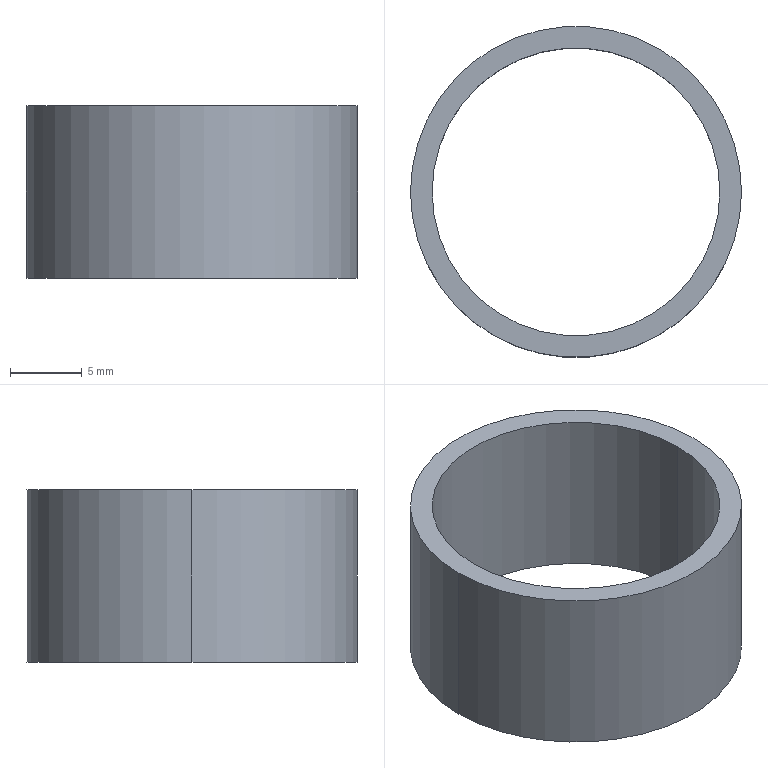Part | SolidWorks | features Extrusion 1 | 1 solid | 6 faces | box 23 x 23 x 12 mm | volume 1216 mm3 | cylinder 4 | plane 2 | commonest cylinder face diameters 20 x2 23 x2
STEP:
#1=CARTESIAN_POINT('',(-10.,0.,12.));
#2=VERTEX_POINT('',#1);
#3=CARTESIAN_POINT('',(10.,0.,12.));
#4=VERTEX_POINT('',#3);
#5=CARTESIAN_POINT('',(0.,0.,12.));
#6=DIRECTION('',(0.,0.,1.));
#7=DIRECTION('',(1.,0.,0.));
#8=AXIS2_PLACEMENT_3D('',#5,#6,#7);
#9=CIRCLE('',#8,10.);
#10=EDGE_CURVE('',#2,#4,#9,.T.);
#11=ORIENTED_EDGE('',*,*,#10,.T.);
#12=CARTESIAN_POINT('',(10.,0.,0.));
#13=VERTEX_POINT('',#12);
#14=CARTESIAN_POINT('',(10.,0.,12.));
#15=DIRECTION('',(0.,0.,-1.));
#16=VECTOR('',#15,1000.);
#17=LINE('',#14,#16);
#18=EDGE_CURVE('',#4,#13,#17,.T.);
#19=ORIENTED_EDGE('',*,*,#18,.T.);
#20=CARTESIAN_POINT('',(-10.,0.,0.));
#21=VERTEX_POINT('',#20);
#22=CARTESIAN_POINT('',(0.,0.,0.));
#23=DIRECTION('',(0.,0.,1.));
#24=DIRECTION('',(1.,0.,0.));
#25=AXIS2_PLACEMENT_3D('',#22,#23,#24);
#26=CIRCLE('',#25,10.);
#27=EDGE_CURVE('',#21,#13,#26,.T.);
#28=ORIENTED_EDGE('',*,*,#27,.F.);
#29=CARTESIAN_POINT('',(-10.,0.,12.));
#30=DIRECTION('',(0.,0.,-1.));
#31=VECTOR('',#30,1000.);
#32=LINE('',#29,#31);
#33=EDGE_CURVE('',#2,#21,#32,.T.);
#34=ORIENTED_EDGE('',*,*,#33,.F.);
#35=EDGE_LOOP('',(#11,#19,#28,#34));
#36=FACE_OUTER_BOUND('',#35,.T.);
#37=CARTESIAN_POINT('',(0.,0.,12.));
#38=DIRECTION('',(0.,0.,-1.));
#39=DIRECTION('',(-1.,0.,0.));
#40=AXIS2_PLACEMENT_3D('',#37,#38,#39);
#41=CYLINDRICAL_SURFACE('',#40,10.);
#42=ADVANCED_FACE('',(#36),#41,.F.);
#43=CARTESIAN_POINT('',(11.5,0.,12.));
#44=VERTEX_POINT('',#43);
#45=CARTESIAN_POINT('',(-11.5,0.,12.));
#46=VERTEX_POINT('',#45);
#47=CARTESIAN_POINT('',(0.,0.,12.));
#48=DIRECTION('',(0.,0.,1.));
#49=DIRECTION('',(1.,0.,0.));
#50=AXIS2_PLACEMENT_3D('',#47,#48,#49);
#51=CIRCLE('',#50,11.5);
#52=EDGE_CURVE('',#44,#46,#51,.T.);
#53=ORIENTED_EDGE('',*,*,#52,.F.);
#54=CARTESIAN_POINT('',(11.5,0.,0.));
#55=VERTEX_POINT('',#54);
#56=CARTESIAN_POINT('',(11.5,0.,12.));
#57=DIRECTION('',(0.,0.,-1.));
#58=VECTOR('',#57,1000.);
#59=LINE('',#56,#58);
#60=EDGE_CURVE('',#44,#55,#59,.T.);
#61=ORIENTED_EDGE('',*,*,#60,.T.);
#62=CARTESIAN_POINT('',(-11.5,0.,0.));
#63=VERTEX_POINT('',#62);
#64=CARTESIAN_POINT('',(0.,0.,0.));
#65=DIRECTION('',(0.,0.,1.));
#66=DIRECTION('',(1.,0.,0.));
#67=AXIS2_PLACEMENT_3D('',#64,#65,#66);
#68=CIRCLE('',#67,11.5);
#69=EDGE_CURVE('',#55,#63,#68,.T.);
#70=ORIENTED_EDGE('',*,*,#69,.T.);
#71=CARTESIAN_POINT('',(-11.5,0.,12.));
#72=DIRECTION('',(0.,0.,-1.));
#73=VECTOR('',#72,1000.);
#74=LINE('',#71,#73);
#75=EDGE_CURVE('',#46,#63,#74,.T.);
#76=ORIENTED_EDGE('',*,*,#75,.F.);
#77=EDGE_LOOP('',(#53,#61,#70,#76));
#78=FACE_OUTER_BOUND('',#77,.T.);
#79=CARTESIAN_POINT('',(0.,0.,12.));
#80=DIRECTION('',(0.,0.,-1.));
#81=DIRECTION('',(-1.,0.,0.));
#82=AXIS2_PLACEMENT_3D('',#79,#80,#81);
#83=CYLINDRICAL_SURFACE('',#82,11.5);
#84=ADVANCED_FACE('',(#78),#83,.T.);
#85=CARTESIAN_POINT('',(0.,0.,12.));
#86=DIRECTION('',(0.,0.,1.));
#87=DIRECTION('',(1.,0.,0.));
#88=AXIS2_PLACEMENT_3D('',#85,#86,#87);
#89=CIRCLE('',#88,11.5);
#90=EDGE_CURVE('',#46,#44,#89,.T.);
#91=ORIENTED_EDGE('',*,*,#90,.T.);
#92=ORIENTED_EDGE('',*,*,#52,.T.);
#93=EDGE_LOOP('',(#91,#92));
#94=FACE_OUTER_BOUND('',#93,.T.);
#95=ORIENTED_EDGE('',*,*,#10,.F.);
#96=CARTESIAN_POINT('',(0.,0.,12.));
#97=DIRECTION('',(0.,0.,1.));
#98=DIRECTION('',(1.,0.,0.));
#99=AXIS2_PLACEMENT_3D('',#96,#97,#98);
#100=CIRCLE('',#99,10.);
#101=EDGE_CURVE('',#4,#2,#100,.T.);
#102=ORIENTED_EDGE('',*,*,#101,.F.);
#103=EDGE_LOOP('',(#95,#102));
#104=FACE_BOUND('',#103,.T.);
#105=CARTESIAN_POINT('',(0.,0.,12.));
#106=DIRECTION('',(0.,0.,1.));
#107=DIRECTION('',(1.,0.,0.));
#108=AXIS2_PLACEMENT_3D('',#105,#106,#107);
#109=PLANE('',#108);
#110=ADVANCED_FACE('',(#94,#104),#109,.T.);
#111=CARTESIAN_POINT('',(0.,0.,0.));
#112=DIRECTION('',(0.,0.,1.));
#113=DIRECTION('',(1.,0.,0.));
#114=AXIS2_PLACEMENT_3D('',#111,#112,#113);
#115=CIRCLE('',#114,11.5);
#116=EDGE_CURVE('',#63,#55,#115,.T.);
#117=ORIENTED_EDGE('',*,*,#116,.F.);
#118=ORIENTED_EDGE('',*,*,#69,.F.);
#119=EDGE_LOOP('',(#117,#118));
#120=FACE_OUTER_BOUND('',#119,.T.);
#121=ORIENTED_EDGE('',*,*,#27,.T.);
#122=CARTESIAN_POINT('',(0.,0.,0.));
#123=DIRECTION('',(0.,0.,1.));
#124=DIRECTION('',(1.,0.,0.));
#125=AXIS2_PLACEMENT_3D('',#122,#123,#124);
#126=CIRCLE('',#125,10.);
#127=EDGE_CURVE('',#13,#21,#126,.T.);
#128=ORIENTED_EDGE('',*,*,#127,.T.);
#129=EDGE_LOOP('',(#121,#128));
#130=FACE_BOUND('',#129,.T.);
#131=CARTESIAN_POINT('',(0.,0.,0.));
#132=DIRECTION('',(0.,0.,1.));
#133=DIRECTION('',(1.,0.,0.));
#134=AXIS2_PLACEMENT_3D('',#131,#132,#133);
#135=PLANE('',#134);
#136=ADVANCED_FACE('',(#120,#130),#135,.F.);
#137=ORIENTED_EDGE('',*,*,#60,.F.);
#138=ORIENTED_EDGE('',*,*,#90,.F.);
#139=ORIENTED_EDGE('',*,*,#75,.T.);
#140=ORIENTED_EDGE('',*,*,#116,.T.);
#141=EDGE_LOOP('',(#137,#138,#139,#140));
#142=FACE_OUTER_BOUND('',#141,.T.);
#143=CARTESIAN_POINT('',(0.,0.,12.));
#144=DIRECTION('',(0.,0.,-1.));
#145=DIRECTION('',(-1.,0.,0.));
#146=AXIS2_PLACEMENT_3D('',#143,#144,#145);
#147=CYLINDRICAL_SURFACE('',#146,11.5);
#148=ADVANCED_FACE('',(#142),#147,.T.);
#149=ORIENTED_EDGE('',*,*,#18,.F.);
#150=ORIENTED_EDGE('',*,*,#101,.T.);
#151=ORIENTED_EDGE('',*,*,#33,.T.);
#152=ORIENTED_EDGE('',*,*,#127,.F.);
#153=EDGE_LOOP('',(#149,#150,#151,#152));
#154=FACE_OUTER_BOUND('',#153,.T.);
#155=CARTESIAN_POINT('',(0.,0.,12.));
#156=DIRECTION('',(0.,0.,-1.));
#157=DIRECTION('',(-1.,0.,0.));
#158=AXIS2_PLACEMENT_3D('',#155,#156,#157);
#159=CYLINDRICAL_SURFACE('',#158,10.);
#160=ADVANCED_FACE('',(#154),#159,.F.);
#161=CLOSED_SHELL('',(#42,#84,#110,#136,#148,#160));
#162=MANIFOLD_SOLID_BREP('',#161);
#163=CARTESIAN_POINT('',(0.,0.,0.));
#164=DIRECTION('',(0.,0.,1.));
#165=DIRECTION('',(1.,0.,0.));
#166=AXIS2_PLACEMENT_3D('',#163,#164,#165);
#167=(LENGTH_UNIT()NAMED_UNIT(*)SI_UNIT(.MILLI.,.METRE.));
#168=UNCERTAINTY_MEASURE_WITH_UNIT(LENGTH_MEASURE(0.00001),#167,'','');
#169=(NAMED_UNIT(*)PLANE_ANGLE_UNIT()SI_UNIT($,.RADIAN.));
#170=(NAMED_UNIT(*)SI_UNIT($,.STERADIAN.)SOLID_ANGLE_UNIT());
#171=(GEOMETRIC_REPRESENTATION_CONTEXT(3)GLOBAL_UNCERTAINTY_ASSIGNED_CONTEXT((#168))GLOBAL_UNIT_ASSIGNED_CONTEXT((#167,#169,#170))REPRESENTATION_CONTEXT('',''));
#172=ADVANCED_BREP_SHAPE_REPRESENTATION('',(#162,#166),#171);